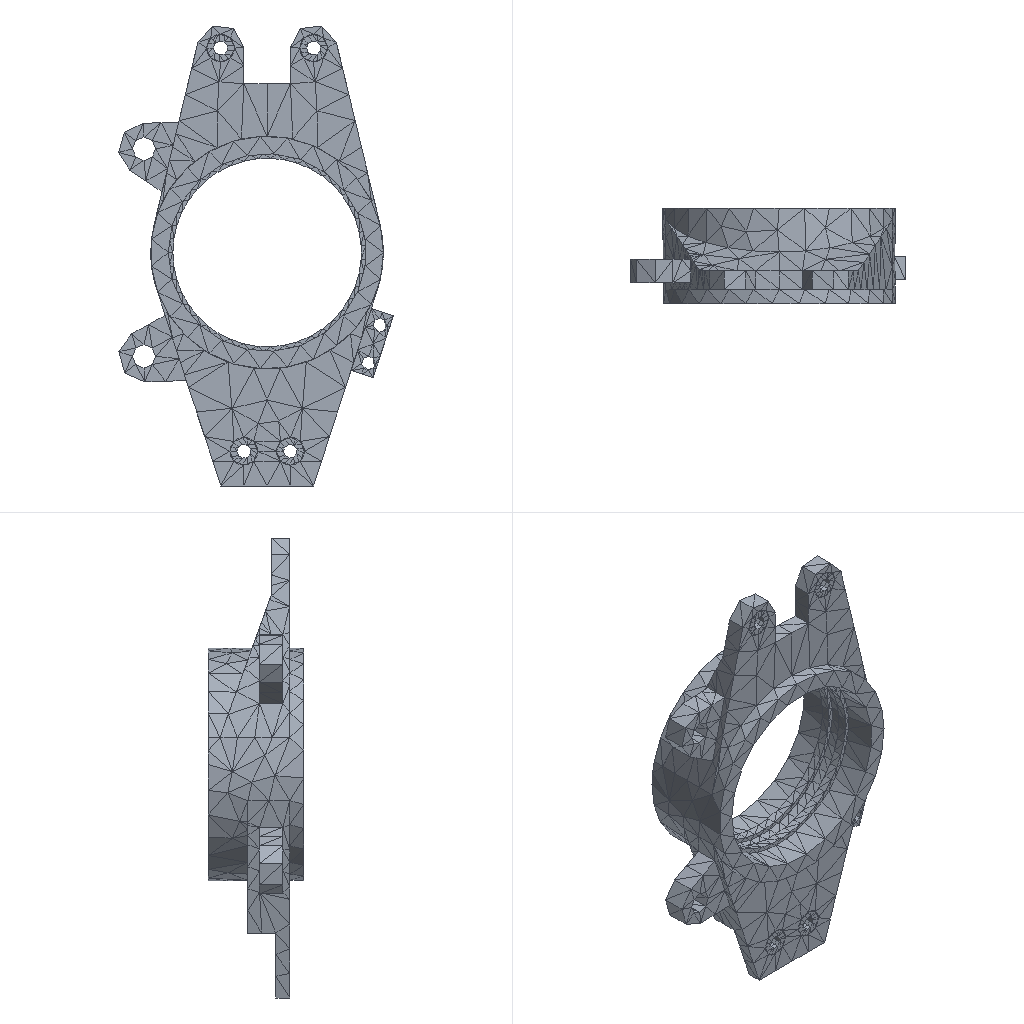Simulation study | ansys workbench
Ansys APDL input file, long lists of numbers shortened:
/batch
/config,noeldb,1     ! force off writing results to database
*get,_wallstrt,active,,time,wall
! ANSYS input file written by Workbench version 2022 R1
! File used for geometry attach:
/title,wbnew--____ (A5)
! ****** Begin Custom Load Command Snippet ******
/COM, ACT Extensions:
/COM,     LSDYNA, 2021.1
/COM,
! ****** End   Custom Load Command Snippet ******
*DIM,_wb_ProjectScratch_dir,string,248
_wb_ProjectScratch_dir(1) = ''
*DIM,_wb_SolverFiles_dir,string,248
_wb_SolverFiles_dir(1) = ''
*DIM,_wb_userfiles_dir,string,248
_wb_userfiles_dir(1) = ''
/com,--- Data in consistent NMM units. See Solving Units in the help system for more information.
/units,MPA
/nopr
/wb,file,start              !  signify a WB generated input file
/prep7
! Turn off shape checking because checks already performed inside WB mesher.
! See help system for more information.
SHPP,OFF,,NOWARN
/nolist
etcon,set             ! allow ANSYS to choose best KEYOP's for 180x elements, resets any applicable keyopt to MAPDL defaults
/com,*********** Nodes for the whole assembly ***********
nblock,3,,8127
(1i9,3e20.9e3)
        1     1.746936171E+01    -8.500785590E+00     8.488039466E+01
! (7388 more lines like these left out)
-1
/wb,elem,start            !  set before creation of elements
/com,*********** Elements for Body 1 "qianzhuan_2025\fix_end 2" ***********
et,1,186
keyo,1,2,1          ! set full integration on SOLID186
eblock,19,solid,,76
(19i9)
        1        1        1        1        0        0        0        0       20        0       77      494      598      597      529      497      632      613      553
! (151 more lines like these left out)
-1
/com,*********** Elements for Body 2 "qianzhuan_2025\fix_end 3" ***********
et,2,186
keyo,2,2,1          ! set full integration on SOLID186
eblock,19,solid,,76
(19i9)
        2        2        2        2        0        0        0        0       20        0        1       55       79       80       56       67      135      134       68
! (151 more lines like these left out)
-1
/com,*********** Elements for Body 3 "qianzhuan_2025\fix_end 4" ***********
et,3,186
keyo,3,2,1          ! set full integration on SOLID186
eblock,19,solid,,57
(19i9)
        3        3        3        3        0        0        0        0       20        0      153     1033     1056     1057     1034     1048     1091     1092     1047
! (113 more lines like these left out)
-1
/com,*********** Elements for Body 4 "qianzhuan_2025\fix_end 1" ***********
et,4,186
keyo,4,2,1          ! set full integration on SOLID186
eblock,19,solid,,57
(19i9)
        4        4        4        4        0        0        0        0       20        0      210     1417     1440     1441     1418     1432     1475     1476     1431
! (113 more lines like these left out)
-1
/com,*********** Elements for Body 5 "qianzhuan_2025\qianzhuan" ***********
et,5,187
eblock,19,solid,,2770
(19i9)
        5        5        5        5        0        0        0        0       10        0      267     1940     1947     1957     2732     3818     3885     3819     3821
! (5539 more lines like these left out)
-1
/wb,elem,end               !  done creating elements
/com,*********** Send User Defined Coordinate System(s) ***********
csys,0
toffst,273.15,  ! Temperature offset from absolute zero
/com,*********** Set Reference Temperature ***********
tref,22.
/wb,mat,start              !  starting to send materials
/com,*********** Send Materials ***********
MP,EX,1,68950,	! tonne s^-2 mm^-1
MP,NUXY,1,0.33,
MP,DENS,1,2.7e-09,	! tonne mm^-3
MP,ALPX,1,7.88860905221012e-31,	! C^-1
! (31 more lines like these left out)
/wb,mat,end                !  done sending materials
!************************* Model Summary ********************
!qianzhuan_2025\fix_end 2,	Aluminum 6061-T6; 6061-T651,	matid,	1
!qianzhuan_2025\fix_end 3,	Aluminum 6061-T6; 6061-T651,	matid,	2
!qianzhuan_2025\fix_end 4,	Aluminum 6061-T6; 6061-T651,	matid,	3
!qianzhuan_2025\fix_end 1,	Aluminum 6061-T6; 6061-T651,	matid,	4
!qianzhuan_2025\qianzhuan,	Aluminum 6061-T6; 6061-T651,	matid,	5
!************************* End Model Summary ********************
! get the diagonal of the bounding box. Needed later for other things
*get,_xmin,node,,mnloc,x
*get,_ymin,node,,mnloc,y
*get,_zmin,node,,mnloc,z
*get,_xmax,node,,mxloc,x
*get,_ymax,node,,mxloc,y
*get,_zmax,node,,mxloc,z
_ASMDIAG=(_xmax-_xmin)*(_xmax-_xmin)+(_ymax-_ymin)*(_ymax-_ymin)+(_zmax-_zmin)*(_zmax-_zmin)
_ASMDIAG=SQRT(_ASMDIAG)
/wb,contact,start          !  starting to send contact
/com,*********** Create Contact "接触区域" ***********
/com,            Real Constant Set For Above Contact Is 7 & 6
*set,tid,7
*set,cid,6
r,tid
r,cid
et,tid,170
et,cid,174
eblock,10,,,68
(15i9)
     5355        7        7        7        0      518      503      614      565      681      683      872      727
! (67 more lines like these left out)
-1
eblock,10,,,68
(15i9)
     5423        6        6        6        0      518      503      614      565      681      683      872      727
! (67 more lines like these left out)
-1
eblock,10,,,16
(15i9)
     5491        6        7        6        0     1806     1809     1820     1820     2991     3013     1820     2995
! (15 more lines like these left out)
-1
eblock,10,,,16
(15i9)
     5507        7        6        7        0     1806     1809     1820     1820     2991     3013     1820     2995
! (15 more lines like these left out)
-1
keyo,cid,8,2               ! auto create asymmetric contact (from Program Controlled setting)
keyo,cid,10,0              ! adjust contact stiffness each NR iteration (from Program Controlled setting)
keyo,cid,12,5              ! bonded always
keyo,cid,18,1              ! small sliding turned on by application
keyo,cid,2,0               ! augmented Lagrange (from Program Controlled setting)
keyo,cid,4,0               ! on Gauss point (from Program Controlled setting)
keyo,cid,9,1               ! ignore initial gaps/penetration
keyo,cid,7,0               ! No Prediction
rmod,tid,3,10.      ! FKN
rmod,tid,5,0.       ! ICONT
rmod,tid,6,0.       ! PINB
rmod,tid,10,0.      ! CNOF
rmod,tid,12,0.      ! FKT
rmod,tid,36,39      ! WB DSID
rmod,cid,3,10.      ! FKN
rmod,cid,5,0.       ! ICONT
rmod,cid,6,0.       ! PINB
rmod,cid,10,0.      ! CNOF
rmod,cid,12,0.      ! FKT
rmod,cid,36,39      ! WB DSID
/com,*********** Create Contact "接触区域 2" ***********
/com,            Real Constant Set For Above Contact Is 9 & 8
*set,tid,9
*set,cid,8
r,tid
r,cid
et,tid,170
et,cid,174
eblock,10,,,68
(15i9)
     5523        9        9        9        0      121      122      123       73      468      470      372      371
! (67 more lines like these left out)
-1
eblock,10,,,68
(15i9)
     5591        8        8        8        0      121      122      123       73      468      470      372      371
! (67 more lines like these left out)
-1
eblock,10,,,16
(15i9)
     5659        8        9        8        0     1790     1793     1800     1800     2910     2930     1800     2912
! (15 more lines like these left out)
-1
eblock,10,,,16
(15i9)
     5675        9        8        9        0     1790     1793     1800     1800     2910     2930     1800     2912
! (15 more lines like these left out)
-1
keyo,cid,8,2               ! auto create asymmetric contact (from Program Controlled setting)
keyo,cid,10,0              ! adjust contact stiffness each NR iteration (from Program Controlled setting)
keyo,cid,12,5              ! bonded always
keyo,cid,18,1              ! small sliding turned on by application
keyo,cid,2,0               ! augmented Lagrange (from Program Controlled setting)
keyo,cid,4,0               ! on Gauss point (from Program Controlled setting)
keyo,cid,9,1               ! ignore initial gaps/penetration
keyo,cid,7,0               ! No Prediction
rmod,tid,3,10.      ! FKN
rmod,tid,5,0.       ! ICONT
rmod,tid,6,0.       ! PINB
rmod,tid,10,0.      ! CNOF
rmod,tid,12,0.      ! FKT
rmod,tid,36,42      ! WB DSID
rmod,cid,3,10.      ! FKN
rmod,cid,5,0.       ! ICONT
rmod,cid,6,0.       ! PINB
rmod,cid,10,0.      ! CNOF
rmod,cid,12,0.      ! FKT
rmod,cid,36,42      ! WB DSID
/com,*********** Create Contact "接触区域 3" ***********
/com,            Real Constant Set For Above Contact Is 11 & 10
*set,tid,11
*set,cid,10
r,tid
r,cid
et,tid,170
et,cid,174
eblock,10,,,51
(15i9)
     5691       11       11       11        0     1082     1083     1084     1050     1354     1356     1291     1290
! (50 more lines like these left out)
-1
eblock,10,,,51
(15i9)
     5742       10       10       10        0     1082     1083     1084     1050     1354     1356     1291     1290
! (50 more lines like these left out)
-1
eblock,10,,,16
(15i9)
     5793       10       11       10        0     1779     1775     1786     1786     2839     2841     1786     2861
! (15 more lines like these left out)
-1
eblock,10,,,16
(15i9)
     5809       11       10       11        0     1779     1775     1786     1786     2839     2841     1786     2861
! (15 more lines like these left out)
-1
keyo,cid,8,2               ! auto create asymmetric contact (from Program Controlled setting)
keyo,cid,10,0              ! adjust contact stiffness each NR iteration (from Program Controlled setting)
keyo,cid,12,5              ! bonded always
keyo,cid,18,1              ! small sliding turned on by application
keyo,cid,2,0               ! augmented Lagrange (from Program Controlled setting)
keyo,cid,4,0               ! on Gauss point (from Program Controlled setting)
keyo,cid,9,1               ! ignore initial gaps/penetration
keyo,cid,7,0               ! No Prediction
rmod,tid,3,10.      ! FKN
rmod,tid,5,0.       ! ICONT
rmod,tid,6,0.       ! PINB
rmod,tid,10,0.      ! CNOF
rmod,tid,12,0.      ! FKT
rmod,tid,36,45      ! WB DSID
rmod,cid,3,10.      ! FKN
rmod,cid,5,0.       ! ICONT
rmod,cid,6,0.       ! PINB
rmod,cid,10,0.      ! CNOF
rmod,cid,12,0.      ! FKT
rmod,cid,36,45      ! WB DSID
/com,*********** Create Contact "接触区域 4" ***********
/com,            Real Constant Set For Above Contact Is 13 & 12
*set,tid,13
*set,cid,12
r,tid
r,cid
et,tid,170
et,cid,174
eblock,10,,,51
(15i9)
     5825       13       13       13        0     1466     1467     1468     1434     1738     1740     1675     1674
! (50 more lines like these left out)
-1
eblock,10,,,51
(15i9)
     5876       12       12       12        0     1466     1467     1468     1434     1738     1740     1675     1674
! (50 more lines like these left out)
-1
eblock,10,,,16
(15i9)
     5927       12       13       12        0     1761     1765     1772     1772     2763     2793     1772     2765
! (15 more lines like these left out)
-1
eblock,10,,,16
(15i9)
     5943       13       12       13        0     1761     1765     1772     1772     2763     2793     1772     2765
! (15 more lines like these left out)
-1
keyo,cid,8,2               ! auto create asymmetric contact (from Program Controlled setting)
keyo,cid,10,0              ! adjust contact stiffness each NR iteration (from Program Controlled setting)
keyo,cid,12,5              ! bonded always
keyo,cid,18,1              ! small sliding turned on by application
keyo,cid,2,0               ! augmented Lagrange (from Program Controlled setting)
keyo,cid,4,0               ! on Gauss point (from Program Controlled setting)
keyo,cid,9,1               ! ignore initial gaps/penetration
keyo,cid,7,0               ! No Prediction
rmod,tid,3,10.      ! FKN
rmod,tid,5,0.       ! ICONT
rmod,tid,6,0.       ! PINB
rmod,tid,10,0.      ! CNOF
rmod,tid,12,0.      ! FKT
rmod,tid,36,48      ! WB DSID
rmod,cid,3,10.      ! FKN
rmod,cid,5,0.       ! ICONT
rmod,cid,6,0.       ! PINB
rmod,cid,10,0.      ! CNOF
rmod,cid,12,0.      ! FKT
rmod,cid,36,48      ! WB DSID
nsel,all
esel,all
/wb,contact,end            !  done creating contacts
/golist
/wb,load,start             !  starting to send loads
/com,*********** Fixed Supports ***********
CMBLOCK,_FIXEDSU,NODE,      670
(8i10)
        28        29        30        31        32        33        34        35
! (83 more lines like these left out)
cmsel,s,_FIXEDSU
d,all,all
nsel,all
/com,*********** Define Force Using Surface Effect Elements ***********
local,12,0,0.,0.,0.,0.,0.,0.
csys,0
et,14,154
eblock,10,,,53
(15i9)
     5959       14       14       14       12     2057     2058     2519     2519     4706     4713     2519     4708
! (52 more lines like these left out)
-1
esel,s,type,,14
keyop,14,2,1                ! Apply load in local coordinate system
keyop,14,7,1                ! Use original area so load is constant in large deformation
esel,all
/gst,on,on
fini
*get,_numnode,node,0,count
*get,_numelem,elem,0,count
*get, _MAXELEMNUM, elem, 0, NUM, MAX
*get, _MAXNODENUM, node, 0, NUM, MAX
*get, _MAXELEMTYPE, etyp, 0, NUM, MAX
*get, _MAXREALCONST, real, 0, NUM, MAX
/go
/wb,load,end               !  done creating loads
/com,--- Number of total nodes = %_numnode%
/com,--- Number of contact elements = 657
/com,--- Number of spring elements = 0
/com,--- Number of bearing elements = 0
/com,--- Number of solid elements = 3036
/com,--- Number of condensed parts = 0
/com,--- Number of total elements = %_numelem%
*get,_wallbsol,active,,time,wall
/com,****************************************************************************
/com,*************************    SOLUTION       ********************************
/com,****************************************************************************
/solu
antype,0                   ! static analysis
_thickRatio=0.2     ! Ratio of thick parts in the model
eqsl,sparse,,,,,1
cntr,print,1               ! print out contact info and also make no initial contact an error
dmpoption,emat,no             ! Don't combine emat file for DANSYS
dmpoption,esav,no             ! Don't combine esav file for DANSYS
nldiag,cont,iter           ! print out contact info each equilibrium iteration
rescontrol,,none                 ! Do not keep any restart files
/com,****************************************************
/com,******************* SOLVE FOR LS 1 OF 1 ****************
esel,s,type,,14
nsle
sfe,all,1,pres,1,-3.50755544878009e-005
sfe,all,2,pres,1,-0.78
sfe,all,3,pres,1,1.75561042254563e-016
nsel,all
esel,all
/nopr
/gopr
nsub,1,1,1
time,1.
outres,erase
outres,all,none
outres,nsol,all,
outres,rsol,all
outres,eangl,all
outres,etmp,all
outres,veng,all
outres,strs,all,
outres,epel,all,
outres,eppl,all,
outres,cont,all,
! *********** WB SOLVE COMMAND ***********
! check interactive state
*get,ANSINTER_,active,,int
*if,ANSINTER_,ne,0,then
/eof
*endif
solve
/com *************** Write FE CONNECTORS *********
CEWRITE,file,ce,,INTE
/com,****************************************************
/com,*************** FINISHED SOLVE FOR LS 1 *************
*get,_wallasol,active,,time,wall
/nopr
*get,_numnode,node,0,count
*get,_numelem,elem,0,count
*get, _MAXELEMNUM, elem, 0, NUM, MAX
*get, _MAXNODENUM, node, 0, NUM, MAX,,,INTERNAL
*get, _MAXELEMTYPE, etyp, 0, NUM, MAX
*get, _MAXREALCONST, real, 0, NUM, MAX
/gopr
/post1
xmlo,ENCODING,ISO-8859-1
xmlo,parm
/xml,parm,xml
fini
/gopr
*get,_walldone,active,,time,wall
_preptime=(_wallbsol-_wallstrt)*3600
_solvtime=(_wallasol-_wallbsol)*3600
_posttime=(_walldone-_wallasol)*3600
_totaltim=(_walldone-_wallstrt)*3600
*get,_dlbratio,active,0,solu,dlbr
*get,_combtime,active,0,solu,comb
*get,_ssmode,active,0,solu,ssmm
*get,_ndofs,active,0,solu,ndof
*get,_sol_end_time,active,0,set,time
*if,_sol_end_time,eq,1.,then
/fclean				!clean distributed files
*endif
/com,--- Total number of nodes = %_numnode%
/com,--- Total number of elements = %_numelem%
/com,--- Element load balance ratio = %_dlbratio%
/com,--- Time to combine distributed files = %_combtime%
/com,--- Sparse memory mode = %_ssmode%
/com,--- Number of DOF = %_ndofs%
/wb,file,end               ! done with WB generated input